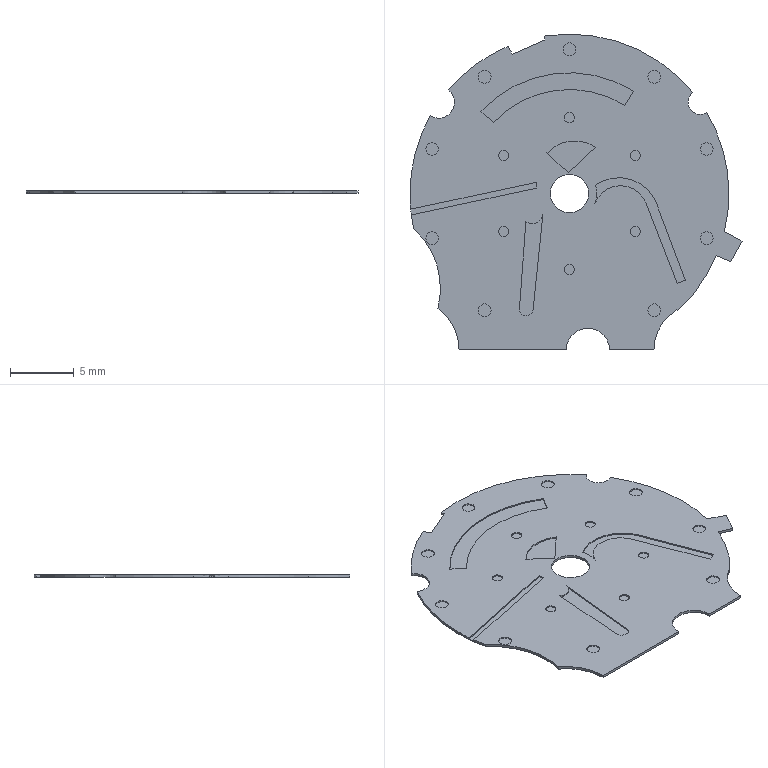Part | SolidWorks | features ICE 4, Extrusion 1 | 1 solid | 97 faces | box 26.026 x 24.754 x 0.2 mm | volume 92.065 mm3 | cylinder 54 | plane 43 | commonest cylinder face diameters 1 x18 0.8 x12 25 x6 1.912 x2 3 x2 4.266 x2